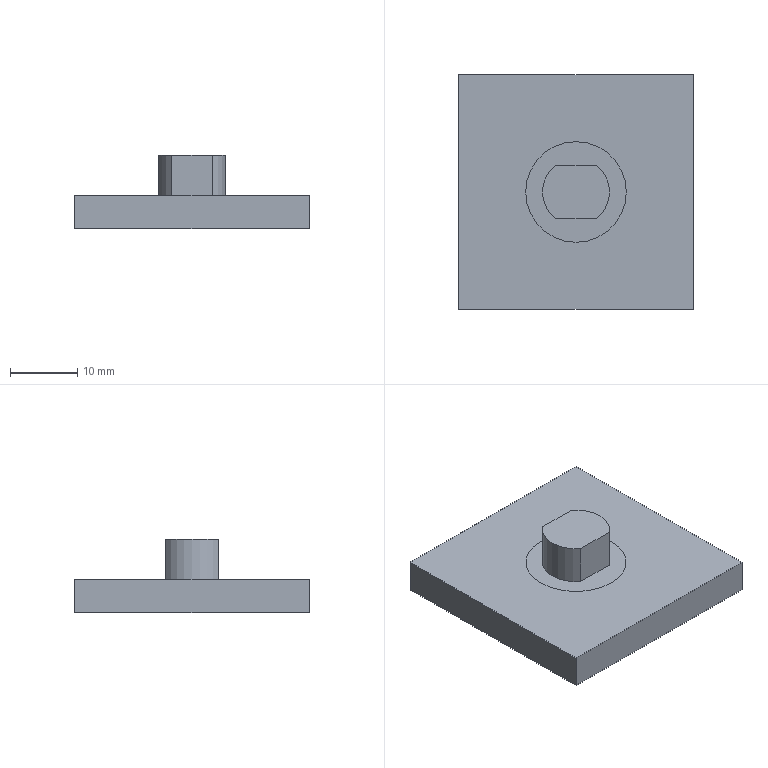Part | NX | 2 solids | 15 faces | box 35 x 35 x 11 mm | volume 6547 mm3 | plane 11 | cylinder 4 | commonest cylinder face diameters 10 x2 15 x2
STEP:
#1=CARTESIAN_POINT('',(-3.,4.,0.));
#2=VERTEX_POINT('',#1);
#3=CARTESIAN_POINT('',(-3.,-4.,0.));
#4=VERTEX_POINT('',#3);
#5=CARTESIAN_POINT('',(0.,0.,0.));
#6=DIRECTION('',(0.,0.,1.));
#7=DIRECTION('',(1.,0.,0.));
#8=AXIS2_PLACEMENT_3D('',#5,#6,#7);
#9=CIRCLE('',#8,5.);
#10=EDGE_CURVE('',#2,#4,#9,.T.);
#11=ORIENTED_EDGE('',*,*,#10,.T.);
#12=CARTESIAN_POINT('',(-3.,-4.,6.));
#13=VERTEX_POINT('',#12);
#14=CARTESIAN_POINT('',(-3.,-4.,6.));
#15=DIRECTION('',(0.,0.,-1.));
#16=VECTOR('',#15,1000.);
#17=LINE('',#14,#16);
#18=EDGE_CURVE('',#13,#4,#17,.T.);
#19=ORIENTED_EDGE('',*,*,#18,.F.);
#20=CARTESIAN_POINT('',(-3.,4.,6.));
#21=VERTEX_POINT('',#20);
#22=CARTESIAN_POINT('',(0.,0.,6.));
#23=DIRECTION('',(0.,0.,1.));
#24=DIRECTION('',(1.,0.,0.));
#25=AXIS2_PLACEMENT_3D('',#22,#23,#24);
#26=CIRCLE('',#25,5.);
#27=EDGE_CURVE('',#21,#13,#26,.T.);
#28=ORIENTED_EDGE('',*,*,#27,.F.);
#29=CARTESIAN_POINT('',(-3.,4.,6.));
#30=DIRECTION('',(0.,0.,-1.));
#31=VECTOR('',#30,1000.);
#32=LINE('',#29,#31);
#33=EDGE_CURVE('',#21,#2,#32,.T.);
#34=ORIENTED_EDGE('',*,*,#33,.T.);
#35=EDGE_LOOP('',(#11,#19,#28,#34));
#36=FACE_BOUND('',#35,.T.);
#37=CARTESIAN_POINT('',(0.,0.,6.));
#38=DIRECTION('',(0.,0.,-1.));
#39=DIRECTION('',(-1.,0.,0.));
#40=AXIS2_PLACEMENT_3D('',#37,#38,#39);
#41=CYLINDRICAL_SURFACE('',#40,5.);
#42=ADVANCED_FACE('',(#36),#41,.T.);
#43=CARTESIAN_POINT('',(3.,-4.,0.));
#44=VERTEX_POINT('',#43);
#45=CARTESIAN_POINT('',(-3.,-4.,0.));
#46=DIRECTION('',(1.,0.,0.));
#47=VECTOR('',#46,1000.);
#48=LINE('',#45,#47);
#49=EDGE_CURVE('',#4,#44,#48,.T.);
#50=ORIENTED_EDGE('',*,*,#49,.T.);
#51=CARTESIAN_POINT('',(3.,-4.,6.));
#52=VERTEX_POINT('',#51);
#53=CARTESIAN_POINT('',(3.,-4.,6.));
#54=DIRECTION('',(0.,0.,-1.));
#55=VECTOR('',#54,1000.);
#56=LINE('',#53,#55);
#57=EDGE_CURVE('',#52,#44,#56,.T.);
#58=ORIENTED_EDGE('',*,*,#57,.F.);
#59=CARTESIAN_POINT('',(-3.,-4.,6.));
#60=DIRECTION('',(1.,0.,0.));
#61=VECTOR('',#60,1000.);
#62=LINE('',#59,#61);
#63=EDGE_CURVE('',#13,#52,#62,.T.);
#64=ORIENTED_EDGE('',*,*,#63,.F.);
#65=ORIENTED_EDGE('',*,*,#18,.T.);
#66=EDGE_LOOP('',(#50,#58,#64,#65));
#67=FACE_BOUND('',#66,.T.);
#68=CARTESIAN_POINT('',(-3.,-4.,6.));
#69=DIRECTION('',(0.,1.,0.));
#70=DIRECTION('',(0.,0.,1.));
#71=AXIS2_PLACEMENT_3D('',#68,#69,#70);
#72=PLANE('',#71);
#73=ADVANCED_FACE('',(#67),#72,.F.);
#74=CARTESIAN_POINT('',(3.,4.,0.));
#75=VERTEX_POINT('',#74);
#76=CARTESIAN_POINT('',(0.,0.,0.));
#77=DIRECTION('',(0.,0.,1.));
#78=DIRECTION('',(1.,0.,0.));
#79=AXIS2_PLACEMENT_3D('',#76,#77,#78);
#80=CIRCLE('',#79,5.);
#81=EDGE_CURVE('',#44,#75,#80,.T.);
#82=ORIENTED_EDGE('',*,*,#81,.T.);
#83=CARTESIAN_POINT('',(3.,4.,6.));
#84=VERTEX_POINT('',#83);
#85=CARTESIAN_POINT('',(3.,4.,6.));
#86=DIRECTION('',(0.,0.,-1.));
#87=VECTOR('',#86,1000.);
#88=LINE('',#85,#87);
#89=EDGE_CURVE('',#84,#75,#88,.T.);
#90=ORIENTED_EDGE('',*,*,#89,.F.);
#91=CARTESIAN_POINT('',(0.,0.,6.));
#92=DIRECTION('',(0.,0.,1.));
#93=DIRECTION('',(1.,0.,0.));
#94=AXIS2_PLACEMENT_3D('',#91,#92,#93);
#95=CIRCLE('',#94,5.);
#96=EDGE_CURVE('',#52,#84,#95,.T.);
#97=ORIENTED_EDGE('',*,*,#96,.F.);
#98=ORIENTED_EDGE('',*,*,#57,.T.);
#99=EDGE_LOOP('',(#82,#90,#97,#98));
#100=FACE_BOUND('',#99,.T.);
#101=CARTESIAN_POINT('',(0.,0.,6.));
#102=DIRECTION('',(0.,0.,-1.));
#103=DIRECTION('',(-1.,0.,0.));
#104=AXIS2_PLACEMENT_3D('',#101,#102,#103);
#105=CYLINDRICAL_SURFACE('',#104,5.);
#106=ADVANCED_FACE('',(#100),#105,.T.);
#107=CARTESIAN_POINT('',(3.,4.,0.));
#108=DIRECTION('',(-1.,0.,0.));
#109=VECTOR('',#108,1000.);
#110=LINE('',#107,#109);
#111=EDGE_CURVE('',#75,#2,#110,.T.);
#112=ORIENTED_EDGE('',*,*,#111,.T.);
#113=ORIENTED_EDGE('',*,*,#33,.F.);
#114=CARTESIAN_POINT('',(3.,4.,6.));
#115=DIRECTION('',(-1.,0.,0.));
#116=VECTOR('',#115,1000.);
#117=LINE('',#114,#116);
#118=EDGE_CURVE('',#84,#21,#117,.T.);
#119=ORIENTED_EDGE('',*,*,#118,.F.);
#120=ORIENTED_EDGE('',*,*,#89,.T.);
#121=EDGE_LOOP('',(#112,#113,#119,#120));
#122=FACE_BOUND('',#121,.T.);
#123=CARTESIAN_POINT('',(3.,4.,6.));
#124=DIRECTION('',(0.,-1.,0.));
#125=DIRECTION('',(0.,0.,-1.));
#126=AXIS2_PLACEMENT_3D('',#123,#124,#125);
#127=PLANE('',#126);
#128=ADVANCED_FACE('',(#122),#127,.F.);
#129=ORIENTED_EDGE('',*,*,#27,.T.);
#130=ORIENTED_EDGE('',*,*,#63,.T.);
#131=ORIENTED_EDGE('',*,*,#96,.T.);
#132=ORIENTED_EDGE('',*,*,#118,.T.);
#133=EDGE_LOOP('',(#129,#130,#131,#132));
#134=FACE_BOUND('',#133,.T.);
#135=CARTESIAN_POINT('',(0.,0.,6.));
#136=DIRECTION('',(0.,0.,1.));
#137=DIRECTION('',(1.,0.,0.));
#138=AXIS2_PLACEMENT_3D('',#135,#136,#137);
#139=PLANE('',#138);
#140=ADVANCED_FACE('',(#134),#139,.T.);
#141=CARTESIAN_POINT('',(7.5,0.,0.));
#142=VERTEX_POINT('',#141);
#143=CARTESIAN_POINT('',(0.,0.,0.));
#144=DIRECTION('',(0.,0.,1.));
#145=DIRECTION('',(1.,0.,0.));
#146=AXIS2_PLACEMENT_3D('',#143,#144,#145);
#147=CIRCLE('',#146,7.5);
#148=EDGE_CURVE('',#142,#142,#147,.T.);
#149=ORIENTED_EDGE('',*,*,#148,.T.);
#150=EDGE_LOOP('',(#149));
#151=FACE_BOUND('',#150,.T.);
#152=ORIENTED_EDGE('',*,*,#10,.F.);
#153=ORIENTED_EDGE('',*,*,#111,.F.);
#154=ORIENTED_EDGE('',*,*,#81,.F.);
#155=ORIENTED_EDGE('',*,*,#49,.F.);
#156=EDGE_LOOP('',(#152,#153,#154,#155));
#157=FACE_BOUND('',#156,.T.);
#158=CARTESIAN_POINT('',(0.,0.,0.));
#159=DIRECTION('',(0.,0.,1.));
#160=DIRECTION('',(1.,0.,0.));
#161=AXIS2_PLACEMENT_3D('',#158,#159,#160);
#162=PLANE('',#161);
#163=ADVANCED_FACE('',(#151,#157),#162,.T.);
#164=CARTESIAN_POINT('',(7.5,0.,-5.));
#165=VERTEX_POINT('',#164);
#166=CARTESIAN_POINT('',(0.,0.,-5.));
#167=DIRECTION('',(0.,0.,1.));
#168=DIRECTION('',(1.,0.,0.));
#169=AXIS2_PLACEMENT_3D('',#166,#167,#168);
#170=CIRCLE('',#169,7.5);
#171=EDGE_CURVE('',#165,#165,#170,.T.);
#172=ORIENTED_EDGE('',*,*,#171,.T.);
#173=EDGE_LOOP('',(#172));
#174=FACE_BOUND('',#173,.T.);
#175=ORIENTED_EDGE('',*,*,#148,.F.);
#176=EDGE_LOOP('',(#175));
#177=FACE_BOUND('',#176,.T.);
#178=CARTESIAN_POINT('',(0.,0.,-5.));
#179=DIRECTION('',(0.,0.,1.));
#180=DIRECTION('',(1.,0.,0.));
#181=AXIS2_PLACEMENT_3D('',#178,#179,#180);
#182=CYLINDRICAL_SURFACE('',#181,7.5);
#183=ADVANCED_FACE('',(#174,#177),#182,.T.);
#184=ORIENTED_EDGE('',*,*,#171,.F.);
#185=EDGE_LOOP('',(#184));
#186=FACE_BOUND('',#185,.T.);
#187=CARTESIAN_POINT('',(0.,0.,-5.));
#188=DIRECTION('',(0.,0.,1.));
#189=DIRECTION('',(1.,0.,0.));
#190=AXIS2_PLACEMENT_3D('',#187,#188,#189);
#191=PLANE('',#190);
#192=ADVANCED_FACE('',(#186),#191,.F.);
#193=CLOSED_SHELL('',(#42,#73,#106,#128,#140,#163,#183,#192));
#194=MANIFOLD_SOLID_BREP('',#193);
#195=CARTESIAN_POINT('',(-17.5,-17.5,-5.));
#196=VERTEX_POINT('',#195);
#197=CARTESIAN_POINT('',(-17.5,17.5,-5.));
#198=VERTEX_POINT('',#197);
#199=CARTESIAN_POINT('',(-17.5,-17.5,-5.));
#200=DIRECTION('',(0.,1.,0.));
#201=VECTOR('',#200,1000.);
#202=LINE('',#199,#201);
#203=EDGE_CURVE('',#196,#198,#202,.T.);
#204=ORIENTED_EDGE('',*,*,#203,.F.);
#205=CARTESIAN_POINT('',(-17.5,-17.5,0.));
#206=VERTEX_POINT('',#205);
#207=CARTESIAN_POINT('',(-17.5,-17.5,0.));
#208=DIRECTION('',(0.,0.,-1.));
#209=VECTOR('',#208,1000.);
#210=LINE('',#207,#209);
#211=EDGE_CURVE('',#206,#196,#210,.T.);
#212=ORIENTED_EDGE('',*,*,#211,.F.);
#213=CARTESIAN_POINT('',(-17.5,17.5,0.));
#214=VERTEX_POINT('',#213);
#215=CARTESIAN_POINT('',(-17.5,-17.5,0.));
#216=DIRECTION('',(0.,1.,0.));
#217=VECTOR('',#216,1000.);
#218=LINE('',#215,#217);
#219=EDGE_CURVE('',#206,#214,#218,.T.);
#220=ORIENTED_EDGE('',*,*,#219,.T.);
#221=CARTESIAN_POINT('',(-17.5,17.5,0.));
#222=DIRECTION('',(0.,0.,-1.));
#223=VECTOR('',#222,1000.);
#224=LINE('',#221,#223);
#225=EDGE_CURVE('',#214,#198,#224,.T.);
#226=ORIENTED_EDGE('',*,*,#225,.T.);
#227=EDGE_LOOP('',(#204,#212,#220,#226));
#228=FACE_BOUND('',#227,.T.);
#229=CARTESIAN_POINT('',(-17.5,-17.5,0.));
#230=DIRECTION('',(-1.,0.,0.));
#231=DIRECTION('',(0.,-1.,0.));
#232=AXIS2_PLACEMENT_3D('',#229,#230,#231);
#233=PLANE('',#232);
#234=ADVANCED_FACE('',(#228),#233,.T.);
#235=CARTESIAN_POINT('',(17.5,17.5,-5.));
#236=VERTEX_POINT('',#235);
#237=CARTESIAN_POINT('',(-17.5,17.5,-5.));
#238=DIRECTION('',(1.,0.,0.));
#239=VECTOR('',#238,1000.);
#240=LINE('',#237,#239);
#241=EDGE_CURVE('',#198,#236,#240,.T.);
#242=ORIENTED_EDGE('',*,*,#241,.F.);
#243=ORIENTED_EDGE('',*,*,#225,.F.);
#244=CARTESIAN_POINT('',(17.5,17.5,0.));
#245=VERTEX_POINT('',#244);
#246=CARTESIAN_POINT('',(-17.5,17.5,0.));
#247=DIRECTION('',(1.,0.,0.));
#248=VECTOR('',#247,1000.);
#249=LINE('',#246,#248);
#250=EDGE_CURVE('',#214,#245,#249,.T.);
#251=ORIENTED_EDGE('',*,*,#250,.T.);
#252=CARTESIAN_POINT('',(17.5,17.5,0.));
#253=DIRECTION('',(0.,0.,-1.));
#254=VECTOR('',#253,1000.);
#255=LINE('',#252,#254);
#256=EDGE_CURVE('',#245,#236,#255,.T.);
#257=ORIENTED_EDGE('',*,*,#256,.T.);
#258=EDGE_LOOP('',(#242,#243,#251,#257));
#259=FACE_BOUND('',#258,.T.);
#260=CARTESIAN_POINT('',(-17.5,17.5,0.));
#261=DIRECTION('',(0.,1.,0.));
#262=DIRECTION('',(-1.,0.,0.));
#263=AXIS2_PLACEMENT_3D('',#260,#261,#262);
#264=PLANE('',#263);
#265=ADVANCED_FACE('',(#259),#264,.T.);
#266=CARTESIAN_POINT('',(17.5,-17.5,-5.));
#267=VERTEX_POINT('',#266);
#268=CARTESIAN_POINT('',(17.5,17.5,-5.));
#269=DIRECTION('',(0.,-1.,0.));
#270=VECTOR('',#269,1000.);
#271=LINE('',#268,#270);
#272=EDGE_CURVE('',#236,#267,#271,.T.);
#273=ORIENTED_EDGE('',*,*,#272,.F.);
#274=ORIENTED_EDGE('',*,*,#256,.F.);
#275=CARTESIAN_POINT('',(17.5,-17.5,0.));
#276=VERTEX_POINT('',#275);
#277=CARTESIAN_POINT('',(17.5,17.5,0.));
#278=DIRECTION('',(0.,-1.,0.));
#279=VECTOR('',#278,1000.);
#280=LINE('',#277,#279);
#281=EDGE_CURVE('',#245,#276,#280,.T.);
#282=ORIENTED_EDGE('',*,*,#281,.T.);
#283=CARTESIAN_POINT('',(17.5,-17.5,0.));
#284=DIRECTION('',(0.,0.,-1.));
#285=VECTOR('',#284,1000.);
#286=LINE('',#283,#285);
#287=EDGE_CURVE('',#276,#267,#286,.T.);
#288=ORIENTED_EDGE('',*,*,#287,.T.);
#289=EDGE_LOOP('',(#273,#274,#282,#288));
#290=FACE_BOUND('',#289,.T.);
#291=CARTESIAN_POINT('',(17.5,17.5,0.));
#292=DIRECTION('',(1.,0.,0.));
#293=DIRECTION('',(0.,1.,0.));
#294=AXIS2_PLACEMENT_3D('',#291,#292,#293);
#295=PLANE('',#294);
#296=ADVANCED_FACE('',(#290),#295,.T.);
#297=CARTESIAN_POINT('',(17.5,-17.5,-5.));
#298=DIRECTION('',(-1.,0.,0.));
#299=VECTOR('',#298,1000.);
#300=LINE('',#297,#299);
#301=EDGE_CURVE('',#267,#196,#300,.T.);
#302=ORIENTED_EDGE('',*,*,#301,.F.);
#303=ORIENTED_EDGE('',*,*,#287,.F.);
#304=CARTESIAN_POINT('',(17.5,-17.5,0.));
#305=DIRECTION('',(-1.,0.,0.));
#306=VECTOR('',#305,1000.);
#307=LINE('',#304,#306);
#308=EDGE_CURVE('',#276,#206,#307,.T.);
#309=ORIENTED_EDGE('',*,*,#308,.T.);
#310=ORIENTED_EDGE('',*,*,#211,.T.);
#311=EDGE_LOOP('',(#302,#303,#309,#310));
#312=FACE_BOUND('',#311,.T.);
#313=CARTESIAN_POINT('',(17.5,-17.5,0.));
#314=DIRECTION('',(0.,-1.,0.));
#315=DIRECTION('',(1.,0.,0.));
#316=AXIS2_PLACEMENT_3D('',#313,#314,#315);
#317=PLANE('',#316);
#318=ADVANCED_FACE('',(#312),#317,.T.);
#319=CARTESIAN_POINT('',(7.5,0.,0.));
#320=VERTEX_POINT('',#319);
#321=CARTESIAN_POINT('',(0.,0.,0.));
#322=DIRECTION('',(0.,0.,-1.));
#323=DIRECTION('',(1.,0.,0.));
#324=AXIS2_PLACEMENT_3D('',#321,#322,#323);
#325=CIRCLE('',#324,7.5);
#326=EDGE_CURVE('',#320,#320,#325,.T.);
#327=ORIENTED_EDGE('',*,*,#326,.F.);
#328=EDGE_LOOP('',(#327));
#329=FACE_BOUND('',#328,.T.);
#330=CARTESIAN_POINT('',(7.5,0.,-5.));
#331=VERTEX_POINT('',#330);
#332=CARTESIAN_POINT('',(0.,0.,-5.));
#333=DIRECTION('',(0.,0.,-1.));
#334=DIRECTION('',(1.,0.,0.));
#335=AXIS2_PLACEMENT_3D('',#332,#333,#334);
#336=CIRCLE('',#335,7.5);
#337=EDGE_CURVE('',#331,#331,#336,.T.);
#338=ORIENTED_EDGE('',*,*,#337,.T.);
#339=EDGE_LOOP('',(#338));
#340=FACE_BOUND('',#339,.T.);
#341=CARTESIAN_POINT('',(0.,0.,0.));
#342=DIRECTION('',(0.,0.,-1.));
#343=DIRECTION('',(-1.,0.,0.));
#344=AXIS2_PLACEMENT_3D('',#341,#342,#343);
#345=CYLINDRICAL_SURFACE('',#344,7.5);
#346=ADVANCED_FACE('',(#329,#340),#345,.F.);
#347=ORIENTED_EDGE('',*,*,#219,.F.);
#348=ORIENTED_EDGE('',*,*,#308,.F.);
#349=ORIENTED_EDGE('',*,*,#281,.F.);
#350=ORIENTED_EDGE('',*,*,#250,.F.);
#351=EDGE_LOOP('',(#347,#348,#349,#350));
#352=FACE_BOUND('',#351,.T.);
#353=ORIENTED_EDGE('',*,*,#326,.T.);
#354=EDGE_LOOP('',(#353));
#355=FACE_BOUND('',#354,.T.);
#356=CARTESIAN_POINT('',(0.,0.,0.));
#357=DIRECTION('',(0.,0.,-1.));
#358=DIRECTION('',(-1.,0.,0.));
#359=AXIS2_PLACEMENT_3D('',#356,#357,#358);
#360=PLANE('',#359);
#361=ADVANCED_FACE('',(#352,#355),#360,.F.);
#362=ORIENTED_EDGE('',*,*,#203,.T.);
#363=ORIENTED_EDGE('',*,*,#241,.T.);
#364=ORIENTED_EDGE('',*,*,#272,.T.);
#365=ORIENTED_EDGE('',*,*,#301,.T.);
#366=EDGE_LOOP('',(#362,#363,#364,#365));
#367=FACE_BOUND('',#366,.T.);
#368=ORIENTED_EDGE('',*,*,#337,.F.);
#369=EDGE_LOOP('',(#368));
#370=FACE_BOUND('',#369,.T.);
#371=CARTESIAN_POINT('',(0.,0.,-5.));
#372=DIRECTION('',(0.,0.,-1.));
#373=DIRECTION('',(-1.,0.,0.));
#374=AXIS2_PLACEMENT_3D('',#371,#372,#373);
#375=PLANE('',#374);
#376=ADVANCED_FACE('',(#367,#370),#375,.T.);
#377=CLOSED_SHELL('',(#234,#265,#296,#318,#346,#361,#376));
#378=MANIFOLD_SOLID_BREP('',#377);
#379=(LENGTH_UNIT()NAMED_UNIT(*)SI_UNIT(.MILLI.,.METRE.));
#380=UNCERTAINTY_MEASURE_WITH_UNIT(LENGTH_MEASURE(0.00001),#379,'','');
#381=(NAMED_UNIT(*)PLANE_ANGLE_UNIT()SI_UNIT($,.RADIAN.));
#382=(NAMED_UNIT(*)SI_UNIT($,.STERADIAN.)SOLID_ANGLE_UNIT());
#383=(GEOMETRIC_REPRESENTATION_CONTEXT(3)GLOBAL_UNCERTAINTY_ASSIGNED_CONTEXT((#380))GLOBAL_UNIT_ASSIGNED_CONTEXT((#379,#381,#382))REPRESENTATION_CONTEXT('',''));
#384=ADVANCED_BREP_SHAPE_REPRESENTATION('',(#194,#378),#383);